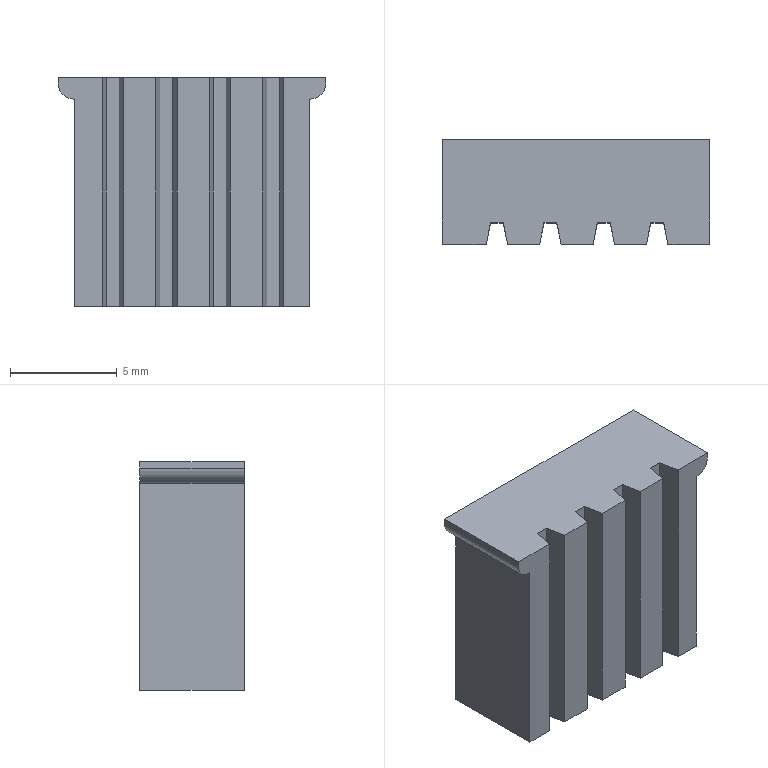Part | STEP file | 0243_105_Sensor_EE-1003 | 1 solid | 28 faces | box 12.5 x 4.9 x 10.7 mm | volume 548.755 mm3 | plane 26 | cylinder 2 | commonest cylinder face diameters 1.4 x2